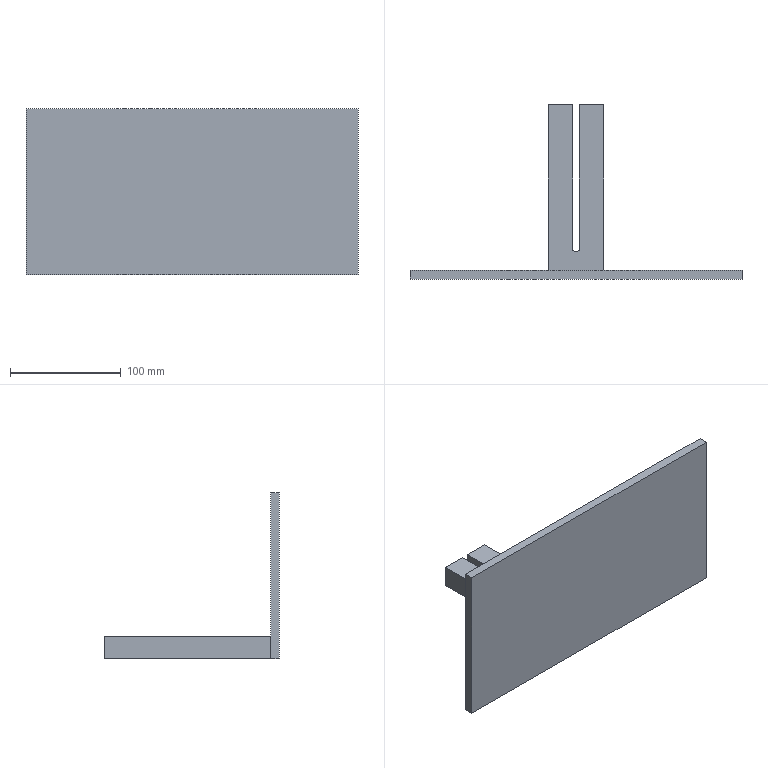Part | SolidWorks | features ICE 2, Extrusion 1 | 1 solid | 14 faces | box 300 x 158 x 150 mm | volume 493578 mm3 | plane 13 | cylinder 1 | commonest cylinder face diameters 6.2 x1
STEP:
#1=CARTESIAN_POINT('',(3.1,158.,-75.));
#2=VERTEX_POINT('',#1);
#3=CARTESIAN_POINT('',(3.1,158.,-55.));
#4=VERTEX_POINT('',#3);
#5=CARTESIAN_POINT('',(3.1,158.,-75.));
#6=DIRECTION('',(0.,0.,1.));
#7=VECTOR('',#6,1000.);
#8=LINE('',#5,#7);
#9=EDGE_CURVE('',#2,#4,#8,.T.);
#10=ORIENTED_EDGE('',*,*,#9,.T.);
#11=CARTESIAN_POINT('',(25.,158.,-55.));
#12=VERTEX_POINT('',#11);
#13=CARTESIAN_POINT('',(-25.,158.,-55.));
#14=DIRECTION('',(1.,0.,0.));
#15=VECTOR('',#14,1000.);
#16=LINE('',#13,#15);
#17=EDGE_CURVE('',#4,#12,#16,.T.);
#18=ORIENTED_EDGE('',*,*,#17,.T.);
#19=CARTESIAN_POINT('',(25.,158.,-75.));
#20=VERTEX_POINT('',#19);
#21=CARTESIAN_POINT('',(25.,158.,-75.));
#22=DIRECTION('',(0.,0.,-1.));
#23=VECTOR('',#22,1000.);
#24=LINE('',#21,#23);
#25=EDGE_CURVE('',#12,#20,#24,.T.);
#26=ORIENTED_EDGE('',*,*,#25,.T.);
#27=CARTESIAN_POINT('',(-25.,158.,-75.));
#28=DIRECTION('',(-1.,0.,0.));
#29=VECTOR('',#28,1000.);
#30=LINE('',#27,#29);
#31=EDGE_CURVE('',#20,#2,#30,.T.);
#32=ORIENTED_EDGE('',*,*,#31,.T.);
#33=EDGE_LOOP('',(#10,#18,#26,#32));
#34=FACE_OUTER_BOUND('',#33,.T.);
#35=CARTESIAN_POINT('',(0.,158.,0.));
#36=DIRECTION('',(0.,1.,0.));
#37=DIRECTION('',(0.,0.,1.));
#38=AXIS2_PLACEMENT_3D('',#35,#36,#37);
#39=PLANE('',#38);
#40=ADVANCED_FACE('',(#34),#39,.T.);
#41=CARTESIAN_POINT('',(-25.,8.,-75.));
#42=VERTEX_POINT('',#41);
#43=CARTESIAN_POINT('',(-25.,8.,-55.));
#44=VERTEX_POINT('',#43);
#45=CARTESIAN_POINT('',(-25.,8.,-75.));
#46=DIRECTION('',(0.,0.,1.));
#47=VECTOR('',#46,1000.);
#48=LINE('',#45,#47);
#49=EDGE_CURVE('',#42,#44,#48,.T.);
#50=ORIENTED_EDGE('',*,*,#49,.F.);
#51=CARTESIAN_POINT('',(-150.,8.,-75.));
#52=VERTEX_POINT('',#51);
#53=CARTESIAN_POINT('',(-150.,8.,-75.));
#54=DIRECTION('',(-1.,0.,0.));
#55=VECTOR('',#54,1000.);
#56=LINE('',#53,#55);
#57=EDGE_CURVE('',#42,#52,#56,.T.);
#58=ORIENTED_EDGE('',*,*,#57,.T.);
#59=CARTESIAN_POINT('',(-150.,8.,75.));
#60=VERTEX_POINT('',#59);
#61=CARTESIAN_POINT('',(-150.,8.,75.));
#62=DIRECTION('',(0.,0.,1.));
#63=VECTOR('',#62,1000.);
#64=LINE('',#61,#63);
#65=EDGE_CURVE('',#52,#60,#64,.T.);
#66=ORIENTED_EDGE('',*,*,#65,.T.);
#67=CARTESIAN_POINT('',(150.,8.,75.));
#68=VERTEX_POINT('',#67);
#69=CARTESIAN_POINT('',(-150.,8.,75.));
#70=DIRECTION('',(1.,0.,0.));
#71=VECTOR('',#70,1000.);
#72=LINE('',#69,#71);
#73=EDGE_CURVE('',#60,#68,#72,.T.);
#74=ORIENTED_EDGE('',*,*,#73,.T.);
#75=CARTESIAN_POINT('',(150.,8.,-75.));
#76=VERTEX_POINT('',#75);
#77=CARTESIAN_POINT('',(150.,8.,75.));
#78=DIRECTION('',(0.,0.,-1.));
#79=VECTOR('',#78,1000.);
#80=LINE('',#77,#79);
#81=EDGE_CURVE('',#68,#76,#80,.T.);
#82=ORIENTED_EDGE('',*,*,#81,.T.);
#83=CARTESIAN_POINT('',(25.,8.,-75.));
#84=VERTEX_POINT('',#83);
#85=CARTESIAN_POINT('',(-150.,8.,-75.));
#86=DIRECTION('',(-1.,0.,0.));
#87=VECTOR('',#86,1000.);
#88=LINE('',#85,#87);
#89=EDGE_CURVE('',#76,#84,#88,.T.);
#90=ORIENTED_EDGE('',*,*,#89,.T.);
#91=CARTESIAN_POINT('',(25.,8.,-55.));
#92=VERTEX_POINT('',#91);
#93=CARTESIAN_POINT('',(25.,8.,-75.));
#94=DIRECTION('',(0.,0.,-1.));
#95=VECTOR('',#94,1000.);
#96=LINE('',#93,#95);
#97=EDGE_CURVE('',#92,#84,#96,.T.);
#98=ORIENTED_EDGE('',*,*,#97,.F.);
#99=CARTESIAN_POINT('',(-25.,8.,-55.));
#100=DIRECTION('',(1.,0.,0.));
#101=VECTOR('',#100,1000.);
#102=LINE('',#99,#101);
#103=EDGE_CURVE('',#44,#92,#102,.T.);
#104=ORIENTED_EDGE('',*,*,#103,.F.);
#105=EDGE_LOOP('',(#50,#58,#66,#74,#82,#90,#98,#104));
#106=FACE_OUTER_BOUND('',#105,.T.);
#107=CARTESIAN_POINT('',(0.,8.,0.));
#108=DIRECTION('',(0.,-1.,0.));
#109=DIRECTION('',(0.,0.,-1.));
#110=AXIS2_PLACEMENT_3D('',#107,#108,#109);
#111=PLANE('',#110);
#112=ADVANCED_FACE('',(#106),#111,.F.);
#113=CARTESIAN_POINT('',(150.,0.,75.));
#114=VERTEX_POINT('',#113);
#115=CARTESIAN_POINT('',(150.,0.,-75.));
#116=VERTEX_POINT('',#115);
#117=CARTESIAN_POINT('',(150.,0.,75.));
#118=DIRECTION('',(0.,0.,-1.));
#119=VECTOR('',#118,1000.);
#120=LINE('',#117,#119);
#121=EDGE_CURVE('',#114,#116,#120,.T.);
#122=ORIENTED_EDGE('',*,*,#121,.T.);
#123=CARTESIAN_POINT('',(150.,8.,-75.));
#124=DIRECTION('',(0.,-1.,0.));
#125=VECTOR('',#124,1000.);
#126=LINE('',#123,#125);
#127=EDGE_CURVE('',#76,#116,#126,.T.);
#128=ORIENTED_EDGE('',*,*,#127,.F.);
#129=ORIENTED_EDGE('',*,*,#81,.F.);
#130=CARTESIAN_POINT('',(150.,8.,75.));
#131=DIRECTION('',(0.,-1.,0.));
#132=VECTOR('',#131,1000.);
#133=LINE('',#130,#132);
#134=EDGE_CURVE('',#68,#114,#133,.T.);
#135=ORIENTED_EDGE('',*,*,#134,.T.);
#136=EDGE_LOOP('',(#122,#128,#129,#135));
#137=FACE_OUTER_BOUND('',#136,.T.);
#138=CARTESIAN_POINT('',(150.,8.,75.));
#139=DIRECTION('',(-1.,0.,0.));
#140=DIRECTION('',(0.,0.,1.));
#141=AXIS2_PLACEMENT_3D('',#138,#139,#140);
#142=PLANE('',#141);
#143=ADVANCED_FACE('',(#137),#142,.F.);
#144=CARTESIAN_POINT('',(-3.1,28.,-75.));
#145=VERTEX_POINT('',#144);
#146=CARTESIAN_POINT('',(3.1,28.,-75.));
#147=VERTEX_POINT('',#146);
#148=CARTESIAN_POINT('',(0.,28.,-75.));
#149=DIRECTION('',(0.,0.,1.));
#150=DIRECTION('',(1.,0.,0.));
#151=AXIS2_PLACEMENT_3D('',#148,#149,#150);
#152=CIRCLE('',#151,3.1);
#153=EDGE_CURVE('',#145,#147,#152,.T.);
#154=ORIENTED_EDGE('',*,*,#153,.T.);
#155=CARTESIAN_POINT('',(3.1,158.,-75.));
#156=DIRECTION('',(0.,1.,0.));
#157=VECTOR('',#156,1000.);
#158=LINE('',#155,#157);
#159=EDGE_CURVE('',#147,#2,#158,.T.);
#160=ORIENTED_EDGE('',*,*,#159,.T.);
#161=ORIENTED_EDGE('',*,*,#31,.F.);
#162=CARTESIAN_POINT('',(25.,158.,-75.));
#163=DIRECTION('',(0.,-1.,0.));
#164=VECTOR('',#163,1000.);
#165=LINE('',#162,#164);
#166=EDGE_CURVE('',#20,#84,#165,.T.);
#167=ORIENTED_EDGE('',*,*,#166,.T.);
#168=ORIENTED_EDGE('',*,*,#89,.F.);
#169=ORIENTED_EDGE('',*,*,#127,.T.);
#170=CARTESIAN_POINT('',(-150.,0.,-75.));
#171=VERTEX_POINT('',#170);
#172=CARTESIAN_POINT('',(-150.,0.,-75.));
#173=DIRECTION('',(-1.,0.,0.));
#174=VECTOR('',#173,1000.);
#175=LINE('',#172,#174);
#176=EDGE_CURVE('',#116,#171,#175,.T.);
#177=ORIENTED_EDGE('',*,*,#176,.T.);
#178=CARTESIAN_POINT('',(-150.,8.,-75.));
#179=DIRECTION('',(0.,-1.,0.));
#180=VECTOR('',#179,1000.);
#181=LINE('',#178,#180);
#182=EDGE_CURVE('',#52,#171,#181,.T.);
#183=ORIENTED_EDGE('',*,*,#182,.F.);
#184=ORIENTED_EDGE('',*,*,#57,.F.);
#185=CARTESIAN_POINT('',(-25.,158.,-75.));
#186=VERTEX_POINT('',#185);
#187=CARTESIAN_POINT('',(-25.,158.,-75.));
#188=DIRECTION('',(0.,-1.,0.));
#189=VECTOR('',#188,1000.);
#190=LINE('',#187,#189);
#191=EDGE_CURVE('',#186,#42,#190,.T.);
#192=ORIENTED_EDGE('',*,*,#191,.F.);
#193=CARTESIAN_POINT('',(-3.1,158.,-75.));
#194=VERTEX_POINT('',#193);
#195=CARTESIAN_POINT('',(-25.,158.,-75.));
#196=DIRECTION('',(-1.,0.,0.));
#197=VECTOR('',#196,1000.);
#198=LINE('',#195,#197);
#199=EDGE_CURVE('',#194,#186,#198,.T.);
#200=ORIENTED_EDGE('',*,*,#199,.F.);
#201=CARTESIAN_POINT('',(-3.1,158.,-75.));
#202=DIRECTION('',(0.,-1.,0.));
#203=VECTOR('',#202,1000.);
#204=LINE('',#201,#203);
#205=EDGE_CURVE('',#194,#145,#204,.T.);
#206=ORIENTED_EDGE('',*,*,#205,.T.);
#207=EDGE_LOOP('',(#154,#160,#161,#167,#168,#169,#177,#183,#184,#192,#200,#206));
#208=FACE_OUTER_BOUND('',#207,.T.);
#209=CARTESIAN_POINT('',(-150.,8.,-75.));
#210=DIRECTION('',(0.,0.,1.));
#211=DIRECTION('',(1.,0.,0.));
#212=AXIS2_PLACEMENT_3D('',#209,#210,#211);
#213=PLANE('',#212);
#214=ADVANCED_FACE('',(#208),#213,.F.);
#215=CARTESIAN_POINT('',(-150.,0.,75.));
#216=VERTEX_POINT('',#215);
#217=CARTESIAN_POINT('',(-150.,0.,75.));
#218=DIRECTION('',(0.,0.,1.));
#219=VECTOR('',#218,1000.);
#220=LINE('',#217,#219);
#221=EDGE_CURVE('',#171,#216,#220,.T.);
#222=ORIENTED_EDGE('',*,*,#221,.T.);
#223=CARTESIAN_POINT('',(-150.,8.,75.));
#224=DIRECTION('',(0.,-1.,0.));
#225=VECTOR('',#224,1000.);
#226=LINE('',#223,#225);
#227=EDGE_CURVE('',#60,#216,#226,.T.);
#228=ORIENTED_EDGE('',*,*,#227,.F.);
#229=ORIENTED_EDGE('',*,*,#65,.F.);
#230=ORIENTED_EDGE('',*,*,#182,.T.);
#231=EDGE_LOOP('',(#222,#228,#229,#230));
#232=FACE_OUTER_BOUND('',#231,.T.);
#233=CARTESIAN_POINT('',(-150.,8.,75.));
#234=DIRECTION('',(1.,0.,0.));
#235=DIRECTION('',(0.,0.,-1.));
#236=AXIS2_PLACEMENT_3D('',#233,#234,#235);
#237=PLANE('',#236);
#238=ADVANCED_FACE('',(#232),#237,.F.);
#239=CARTESIAN_POINT('',(-150.,0.,75.));
#240=DIRECTION('',(1.,0.,0.));
#241=VECTOR('',#240,1000.);
#242=LINE('',#239,#241);
#243=EDGE_CURVE('',#216,#114,#242,.T.);
#244=ORIENTED_EDGE('',*,*,#243,.T.);
#245=ORIENTED_EDGE('',*,*,#134,.F.);
#246=ORIENTED_EDGE('',*,*,#73,.F.);
#247=ORIENTED_EDGE('',*,*,#227,.T.);
#248=EDGE_LOOP('',(#244,#245,#246,#247));
#249=FACE_OUTER_BOUND('',#248,.T.);
#250=CARTESIAN_POINT('',(-150.,8.,75.));
#251=DIRECTION('',(0.,0.,-1.));
#252=DIRECTION('',(-1.,0.,0.));
#253=AXIS2_PLACEMENT_3D('',#250,#251,#252);
#254=PLANE('',#253);
#255=ADVANCED_FACE('',(#249),#254,.F.);
#256=ORIENTED_EDGE('',*,*,#121,.F.);
#257=ORIENTED_EDGE('',*,*,#243,.F.);
#258=ORIENTED_EDGE('',*,*,#221,.F.);
#259=ORIENTED_EDGE('',*,*,#176,.F.);
#260=EDGE_LOOP('',(#256,#257,#258,#259));
#261=FACE_OUTER_BOUND('',#260,.T.);
#262=CARTESIAN_POINT('',(0.,0.,0.));
#263=DIRECTION('',(0.,-1.,0.));
#264=DIRECTION('',(0.,0.,-1.));
#265=AXIS2_PLACEMENT_3D('',#262,#263,#264);
#266=PLANE('',#265);
#267=ADVANCED_FACE('',(#261),#266,.T.);
#268=ORIENTED_EDGE('',*,*,#49,.T.);
#269=CARTESIAN_POINT('',(-25.,158.,-55.));
#270=VERTEX_POINT('',#269);
#271=CARTESIAN_POINT('',(-25.,158.,-55.));
#272=DIRECTION('',(0.,-1.,0.));
#273=VECTOR('',#272,1000.);
#274=LINE('',#271,#273);
#275=EDGE_CURVE('',#270,#44,#274,.T.);
#276=ORIENTED_EDGE('',*,*,#275,.F.);
#277=CARTESIAN_POINT('',(-25.,158.,-75.));
#278=DIRECTION('',(0.,0.,1.));
#279=VECTOR('',#278,1000.);
#280=LINE('',#277,#279);
#281=EDGE_CURVE('',#186,#270,#280,.T.);
#282=ORIENTED_EDGE('',*,*,#281,.F.);
#283=ORIENTED_EDGE('',*,*,#191,.T.);
#284=EDGE_LOOP('',(#268,#276,#282,#283));
#285=FACE_OUTER_BOUND('',#284,.T.);
#286=CARTESIAN_POINT('',(-25.,158.,-75.));
#287=DIRECTION('',(1.,0.,0.));
#288=DIRECTION('',(0.,0.,-1.));
#289=AXIS2_PLACEMENT_3D('',#286,#287,#288);
#290=PLANE('',#289);
#291=ADVANCED_FACE('',(#285),#290,.F.);
#292=ORIENTED_EDGE('',*,*,#17,.F.);
#293=CARTESIAN_POINT('',(3.1,28.,-55.));
#294=VERTEX_POINT('',#293);
#295=CARTESIAN_POINT('',(3.1,158.,-55.));
#296=DIRECTION('',(0.,1.,0.));
#297=VECTOR('',#296,1000.);
#298=LINE('',#295,#297);
#299=EDGE_CURVE('',#294,#4,#298,.T.);
#300=ORIENTED_EDGE('',*,*,#299,.F.);
#301=CARTESIAN_POINT('',(-3.1,28.,-55.));
#302=VERTEX_POINT('',#301);
#303=CARTESIAN_POINT('',(0.,28.,-55.));
#304=DIRECTION('',(0.,0.,1.));
#305=DIRECTION('',(1.,0.,0.));
#306=AXIS2_PLACEMENT_3D('',#303,#304,#305);
#307=CIRCLE('',#306,3.1);
#308=EDGE_CURVE('',#302,#294,#307,.T.);
#309=ORIENTED_EDGE('',*,*,#308,.F.);
#310=CARTESIAN_POINT('',(-3.1,158.,-55.));
#311=VERTEX_POINT('',#310);
#312=CARTESIAN_POINT('',(-3.1,158.,-55.));
#313=DIRECTION('',(0.,-1.,0.));
#314=VECTOR('',#313,1000.);
#315=LINE('',#312,#314);
#316=EDGE_CURVE('',#311,#302,#315,.T.);
#317=ORIENTED_EDGE('',*,*,#316,.F.);
#318=CARTESIAN_POINT('',(-25.,158.,-55.));
#319=DIRECTION('',(1.,0.,0.));
#320=VECTOR('',#319,1000.);
#321=LINE('',#318,#320);
#322=EDGE_CURVE('',#270,#311,#321,.T.);
#323=ORIENTED_EDGE('',*,*,#322,.F.);
#324=ORIENTED_EDGE('',*,*,#275,.T.);
#325=ORIENTED_EDGE('',*,*,#103,.T.);
#326=CARTESIAN_POINT('',(25.,158.,-55.));
#327=DIRECTION('',(0.,-1.,0.));
#328=VECTOR('',#327,1000.);
#329=LINE('',#326,#328);
#330=EDGE_CURVE('',#12,#92,#329,.T.);
#331=ORIENTED_EDGE('',*,*,#330,.F.);
#332=EDGE_LOOP('',(#292,#300,#309,#317,#323,#324,#325,#331));
#333=FACE_OUTER_BOUND('',#332,.T.);
#334=CARTESIAN_POINT('',(-25.,158.,-55.));
#335=DIRECTION('',(0.,0.,-1.));
#336=DIRECTION('',(-1.,0.,0.));
#337=AXIS2_PLACEMENT_3D('',#334,#335,#336);
#338=PLANE('',#337);
#339=ADVANCED_FACE('',(#333),#338,.F.);
#340=ORIENTED_EDGE('',*,*,#97,.T.);
#341=ORIENTED_EDGE('',*,*,#166,.F.);
#342=ORIENTED_EDGE('',*,*,#25,.F.);
#343=ORIENTED_EDGE('',*,*,#330,.T.);
#344=EDGE_LOOP('',(#340,#341,#342,#343));
#345=FACE_OUTER_BOUND('',#344,.T.);
#346=CARTESIAN_POINT('',(25.,158.,-75.));
#347=DIRECTION('',(-1.,0.,0.));
#348=DIRECTION('',(0.,0.,1.));
#349=AXIS2_PLACEMENT_3D('',#346,#347,#348);
#350=PLANE('',#349);
#351=ADVANCED_FACE('',(#345),#350,.F.);
#352=CARTESIAN_POINT('',(-3.1,158.,-75.));
#353=DIRECTION('',(0.,0.,1.));
#354=VECTOR('',#353,1000.);
#355=LINE('',#352,#354);
#356=EDGE_CURVE('',#194,#311,#355,.T.);
#357=ORIENTED_EDGE('',*,*,#356,.F.);
#358=ORIENTED_EDGE('',*,*,#199,.T.);
#359=ORIENTED_EDGE('',*,*,#281,.T.);
#360=ORIENTED_EDGE('',*,*,#322,.T.);
#361=EDGE_LOOP('',(#357,#358,#359,#360));
#362=FACE_OUTER_BOUND('',#361,.T.);
#363=CARTESIAN_POINT('',(0.,158.,0.));
#364=DIRECTION('',(0.,1.,0.));
#365=DIRECTION('',(0.,0.,1.));
#366=AXIS2_PLACEMENT_3D('',#363,#364,#365);
#367=PLANE('',#366);
#368=ADVANCED_FACE('',(#362),#367,.T.);
#369=ORIENTED_EDGE('',*,*,#299,.T.);
#370=ORIENTED_EDGE('',*,*,#9,.F.);
#371=ORIENTED_EDGE('',*,*,#159,.F.);
#372=CARTESIAN_POINT('',(3.1,28.,-75.));
#373=DIRECTION('',(0.,0.,1.));
#374=VECTOR('',#373,1000.);
#375=LINE('',#372,#374);
#376=EDGE_CURVE('',#147,#294,#375,.T.);
#377=ORIENTED_EDGE('',*,*,#376,.T.);
#378=EDGE_LOOP('',(#369,#370,#371,#377));
#379=FACE_OUTER_BOUND('',#378,.T.);
#380=CARTESIAN_POINT('',(3.1,158.,-75.));
#381=DIRECTION('',(1.,0.,0.));
#382=DIRECTION('',(0.,1.,0.));
#383=AXIS2_PLACEMENT_3D('',#380,#381,#382);
#384=PLANE('',#383);
#385=ADVANCED_FACE('',(#379),#384,.F.);
#386=ORIENTED_EDGE('',*,*,#308,.T.);
#387=ORIENTED_EDGE('',*,*,#376,.F.);
#388=ORIENTED_EDGE('',*,*,#153,.F.);
#389=CARTESIAN_POINT('',(-3.1,28.,-75.));
#390=DIRECTION('',(0.,0.,1.));
#391=VECTOR('',#390,1000.);
#392=LINE('',#389,#391);
#393=EDGE_CURVE('',#145,#302,#392,.T.);
#394=ORIENTED_EDGE('',*,*,#393,.T.);
#395=EDGE_LOOP('',(#386,#387,#388,#394));
#396=FACE_OUTER_BOUND('',#395,.T.);
#397=CARTESIAN_POINT('',(0.,28.,-75.));
#398=DIRECTION('',(0.,0.,1.));
#399=DIRECTION('',(1.,0.,0.));
#400=AXIS2_PLACEMENT_3D('',#397,#398,#399);
#401=CYLINDRICAL_SURFACE('',#400,3.1);
#402=ADVANCED_FACE('',(#396),#401,.F.);
#403=ORIENTED_EDGE('',*,*,#316,.T.);
#404=ORIENTED_EDGE('',*,*,#393,.F.);
#405=ORIENTED_EDGE('',*,*,#205,.F.);
#406=ORIENTED_EDGE('',*,*,#356,.T.);
#407=EDGE_LOOP('',(#403,#404,#405,#406));
#408=FACE_OUTER_BOUND('',#407,.T.);
#409=CARTESIAN_POINT('',(-3.1,158.,-75.));
#410=DIRECTION('',(-1.,0.,0.));
#411=DIRECTION('',(0.,-1.,0.));
#412=AXIS2_PLACEMENT_3D('',#409,#410,#411);
#413=PLANE('',#412);
#414=ADVANCED_FACE('',(#408),#413,.F.);
#415=CLOSED_SHELL('',(#40,#112,#143,#214,#238,#255,#267,#291,#339,#351,#368,#385,#402,#414));
#416=MANIFOLD_SOLID_BREP('',#415);
#417=CARTESIAN_POINT('',(0.,0.,0.));
#418=DIRECTION('',(0.,0.,1.));
#419=DIRECTION('',(1.,0.,0.));
#420=AXIS2_PLACEMENT_3D('',#417,#418,#419);
#421=(LENGTH_UNIT()NAMED_UNIT(*)SI_UNIT(.MILLI.,.METRE.));
#422=UNCERTAINTY_MEASURE_WITH_UNIT(LENGTH_MEASURE(0.00001),#421,'','');
#423=(NAMED_UNIT(*)PLANE_ANGLE_UNIT()SI_UNIT($,.RADIAN.));
#424=(NAMED_UNIT(*)SI_UNIT($,.STERADIAN.)SOLID_ANGLE_UNIT());
#425=(GEOMETRIC_REPRESENTATION_CONTEXT(3)GLOBAL_UNCERTAINTY_ASSIGNED_CONTEXT((#422))GLOBAL_UNIT_ASSIGNED_CONTEXT((#421,#423,#424))REPRESENTATION_CONTEXT('',''));
#426=ADVANCED_BREP_SHAPE_REPRESENTATION('',(#416,#420),#425);